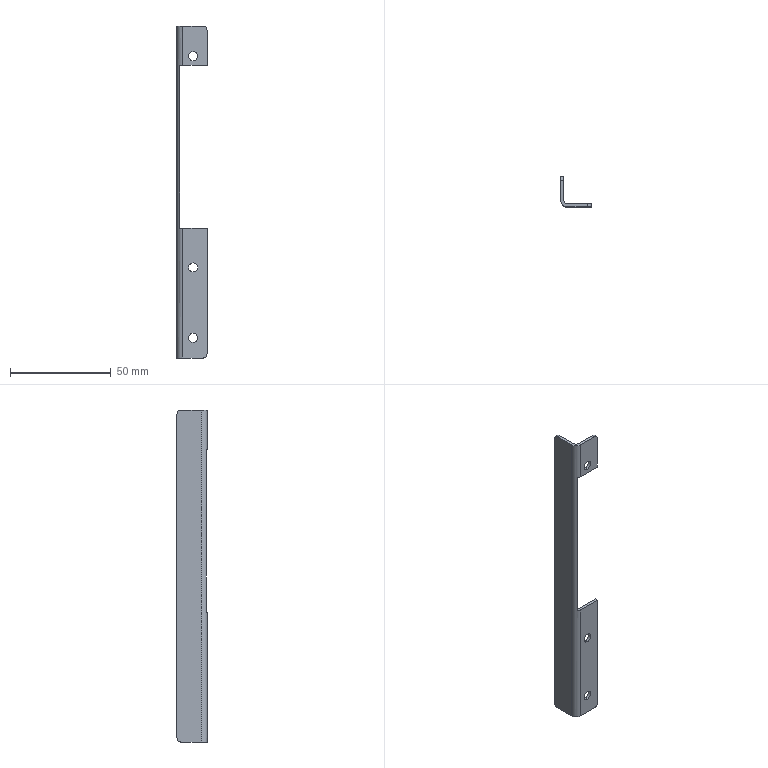Part | STEP file | 229H151431 Default | 1 solid | 26 faces | box 15 x 15 x 165 mm | volume 5074 mm3 | cylinder 13 | plane 13 | commonest cylinder face diameters 4.5 x6 4 x4 3 x2 6 x1
STEP:
#1=CARTESIAN_POINT('',(8.,0.,147.75));
#2=VERTEX_POINT('',#1);
#3=CARTESIAN_POINT('',(8.,0.,152.25));
#4=VERTEX_POINT('',#3);
#5=CARTESIAN_POINT('',(8.,0.,150.));
#6=DIRECTION('',(0.,1.,0.));
#7=DIRECTION('',(0.,0.,1.));
#8=AXIS2_PLACEMENT_3D('',#5,#6,#7);
#9=CIRCLE('',#8,2.25);
#10=EDGE_CURVE('',#2,#4,#9,.T.);
#11=ORIENTED_EDGE('',*,*,#10,.F.);
#12=CARTESIAN_POINT('',(8.,1.5,147.75));
#13=VERTEX_POINT('',#12);
#14=CARTESIAN_POINT('',(8.,-8.5,147.75));
#15=DIRECTION('',(0.,1.,0.));
#16=VECTOR('',#15,1000.);
#17=LINE('',#14,#16);
#18=EDGE_CURVE('',#2,#13,#17,.T.);
#19=ORIENTED_EDGE('',*,*,#18,.T.);
#20=CARTESIAN_POINT('',(8.,1.5,152.25));
#21=VERTEX_POINT('',#20);
#22=CARTESIAN_POINT('',(8.,1.5,150.));
#23=DIRECTION('',(0.,1.,0.));
#24=DIRECTION('',(0.,0.,1.));
#25=AXIS2_PLACEMENT_3D('',#22,#23,#24);
#26=CIRCLE('',#25,2.25);
#27=EDGE_CURVE('',#13,#21,#26,.T.);
#28=ORIENTED_EDGE('',*,*,#27,.T.);
#29=CARTESIAN_POINT('',(8.,-8.5,152.25));
#30=DIRECTION('',(0.,1.,0.));
#31=VECTOR('',#30,1000.);
#32=LINE('',#29,#31);
#33=EDGE_CURVE('',#4,#21,#32,.T.);
#34=ORIENTED_EDGE('',*,*,#33,.F.);
#35=EDGE_LOOP('',(#11,#19,#28,#34));
#36=FACE_OUTER_BOUND('',#35,.T.);
#37=CARTESIAN_POINT('',(8.,-8.5,150.));
#38=DIRECTION('',(0.,1.,0.));
#39=DIRECTION('',(0.,0.,1.));
#40=AXIS2_PLACEMENT_3D('',#37,#38,#39);
#41=CYLINDRICAL_SURFACE('',#40,2.25);
#42=ADVANCED_FACE('',(#36),#41,.F.);
#43=CARTESIAN_POINT('',(8.,0.,42.75));
#44=VERTEX_POINT('',#43);
#45=CARTESIAN_POINT('',(8.,0.,47.25));
#46=VERTEX_POINT('',#45);
#47=CARTESIAN_POINT('',(8.,0.,45.));
#48=DIRECTION('',(0.,1.,0.));
#49=DIRECTION('',(0.,0.,1.));
#50=AXIS2_PLACEMENT_3D('',#47,#48,#49);
#51=CIRCLE('',#50,2.25);
#52=EDGE_CURVE('',#44,#46,#51,.T.);
#53=ORIENTED_EDGE('',*,*,#52,.F.);
#54=CARTESIAN_POINT('',(8.,1.5,42.75));
#55=VERTEX_POINT('',#54);
#56=CARTESIAN_POINT('',(8.,-8.5,42.75));
#57=DIRECTION('',(0.,1.,0.));
#58=VECTOR('',#57,1000.);
#59=LINE('',#56,#58);
#60=EDGE_CURVE('',#44,#55,#59,.T.);
#61=ORIENTED_EDGE('',*,*,#60,.T.);
#62=CARTESIAN_POINT('',(8.,1.5,47.25));
#63=VERTEX_POINT('',#62);
#64=CARTESIAN_POINT('',(8.,1.5,45.));
#65=DIRECTION('',(0.,1.,0.));
#66=DIRECTION('',(0.,0.,1.));
#67=AXIS2_PLACEMENT_3D('',#64,#65,#66);
#68=CIRCLE('',#67,2.25);
#69=EDGE_CURVE('',#55,#63,#68,.T.);
#70=ORIENTED_EDGE('',*,*,#69,.T.);
#71=CARTESIAN_POINT('',(8.,-8.5,47.25));
#72=DIRECTION('',(0.,1.,0.));
#73=VECTOR('',#72,1000.);
#74=LINE('',#71,#73);
#75=EDGE_CURVE('',#46,#63,#74,.T.);
#76=ORIENTED_EDGE('',*,*,#75,.F.);
#77=EDGE_LOOP('',(#53,#61,#70,#76));
#78=FACE_OUTER_BOUND('',#77,.T.);
#79=CARTESIAN_POINT('',(8.,-8.5,45.));
#80=DIRECTION('',(0.,1.,0.));
#81=DIRECTION('',(0.,0.,1.));
#82=AXIS2_PLACEMENT_3D('',#79,#80,#81);
#83=CYLINDRICAL_SURFACE('',#82,2.25);
#84=ADVANCED_FACE('',(#78),#83,.F.);
#85=CARTESIAN_POINT('',(8.,0.,7.75));
#86=VERTEX_POINT('',#85);
#87=CARTESIAN_POINT('',(8.,0.,12.25));
#88=VERTEX_POINT('',#87);
#89=CARTESIAN_POINT('',(8.,0.,10.));
#90=DIRECTION('',(0.,1.,0.));
#91=DIRECTION('',(0.,0.,1.));
#92=AXIS2_PLACEMENT_3D('',#89,#90,#91);
#93=CIRCLE('',#92,2.25);
#94=EDGE_CURVE('',#86,#88,#93,.T.);
#95=ORIENTED_EDGE('',*,*,#94,.F.);
#96=CARTESIAN_POINT('',(8.,1.5,7.75));
#97=VERTEX_POINT('',#96);
#98=CARTESIAN_POINT('',(8.,-8.5,7.75));
#99=DIRECTION('',(0.,1.,0.));
#100=VECTOR('',#99,1000.);
#101=LINE('',#98,#100);
#102=EDGE_CURVE('',#86,#97,#101,.T.);
#103=ORIENTED_EDGE('',*,*,#102,.T.);
#104=CARTESIAN_POINT('',(8.,1.5,12.25));
#105=VERTEX_POINT('',#104);
#106=CARTESIAN_POINT('',(8.,1.5,10.));
#107=DIRECTION('',(0.,1.,0.));
#108=DIRECTION('',(0.,0.,1.));
#109=AXIS2_PLACEMENT_3D('',#106,#107,#108);
#110=CIRCLE('',#109,2.25);
#111=EDGE_CURVE('',#97,#105,#110,.T.);
#112=ORIENTED_EDGE('',*,*,#111,.T.);
#113=CARTESIAN_POINT('',(8.,-8.5,12.25));
#114=DIRECTION('',(0.,1.,0.));
#115=VECTOR('',#114,1000.);
#116=LINE('',#113,#115);
#117=EDGE_CURVE('',#88,#105,#116,.T.);
#118=ORIENTED_EDGE('',*,*,#117,.F.);
#119=EDGE_LOOP('',(#95,#103,#112,#118));
#120=FACE_OUTER_BOUND('',#119,.T.);
#121=CARTESIAN_POINT('',(8.,-8.5,10.));
#122=DIRECTION('',(0.,1.,0.));
#123=DIRECTION('',(0.,0.,1.));
#124=AXIS2_PLACEMENT_3D('',#121,#122,#123);
#125=CYLINDRICAL_SURFACE('',#124,2.25);
#126=ADVANCED_FACE('',(#120),#125,.F.);
#127=CARTESIAN_POINT('',(8.,0.,10.));
#128=DIRECTION('',(0.,1.,0.));
#129=DIRECTION('',(0.,0.,1.));
#130=AXIS2_PLACEMENT_3D('',#127,#128,#129);
#131=CIRCLE('',#130,2.25);
#132=EDGE_CURVE('',#88,#86,#131,.T.);
#133=ORIENTED_EDGE('',*,*,#132,.T.);
#134=ORIENTED_EDGE('',*,*,#94,.T.);
#135=EDGE_LOOP('',(#133,#134));
#136=FACE_BOUND('',#135,.T.);
#137=CARTESIAN_POINT('',(8.,0.,45.));
#138=DIRECTION('',(0.,1.,0.));
#139=DIRECTION('',(0.,0.,1.));
#140=AXIS2_PLACEMENT_3D('',#137,#138,#139);
#141=CIRCLE('',#140,2.25);
#142=EDGE_CURVE('',#46,#44,#141,.T.);
#143=ORIENTED_EDGE('',*,*,#142,.T.);
#144=ORIENTED_EDGE('',*,*,#52,.T.);
#145=EDGE_LOOP('',(#143,#144));
#146=FACE_BOUND('',#145,.T.);
#147=CARTESIAN_POINT('',(15.,0.,64.5));
#148=VERTEX_POINT('',#147);
#149=CARTESIAN_POINT('',(15.,0.,2.));
#150=VERTEX_POINT('',#149);
#151=CARTESIAN_POINT('',(15.,0.,165.));
#152=DIRECTION('',(0.,0.,-1.));
#153=VECTOR('',#152,1000.);
#154=LINE('',#151,#153);
#155=EDGE_CURVE('',#148,#150,#154,.T.);
#156=ORIENTED_EDGE('',*,*,#155,.F.);
#157=CARTESIAN_POINT('',(3.,0.,64.5));
#158=VERTEX_POINT('',#157);
#159=CARTESIAN_POINT('',(0.,0.,64.5));
#160=DIRECTION('',(-1.,0.,0.));
#161=VECTOR('',#160,1000.);
#162=LINE('',#159,#161);
#163=EDGE_CURVE('',#148,#158,#162,.T.);
#164=ORIENTED_EDGE('',*,*,#163,.T.);
#165=CARTESIAN_POINT('',(3.,0.,0.));
#166=VERTEX_POINT('',#165);
#167=CARTESIAN_POINT('',(3.,0.,165.));
#168=DIRECTION('',(0.,0.,-1.));
#169=VECTOR('',#168,1000.);
#170=LINE('',#167,#169);
#171=EDGE_CURVE('',#158,#166,#170,.T.);
#172=ORIENTED_EDGE('',*,*,#171,.T.);
#173=CARTESIAN_POINT('',(13.,0.,0.));
#174=VERTEX_POINT('',#173);
#175=CARTESIAN_POINT('',(0.,0.,0.));
#176=DIRECTION('',(1.,0.,0.));
#177=VECTOR('',#176,1000.);
#178=LINE('',#175,#177);
#179=EDGE_CURVE('',#166,#174,#178,.T.);
#180=ORIENTED_EDGE('',*,*,#179,.T.);
#181=CARTESIAN_POINT('',(13.,0.,2.));
#182=DIRECTION('',(0.,-1.,0.));
#183=DIRECTION('',(0.,0.,1.));
#184=AXIS2_PLACEMENT_3D('',#181,#182,#183);
#185=CIRCLE('',#184,2.);
#186=EDGE_CURVE('',#174,#150,#185,.T.);
#187=ORIENTED_EDGE('',*,*,#186,.T.);
#188=EDGE_LOOP('',(#156,#164,#172,#180,#187));
#189=FACE_OUTER_BOUND('',#188,.T.);
#190=CARTESIAN_POINT('',(0.,0.,165.));
#191=DIRECTION('',(0.,1.,0.));
#192=DIRECTION('',(0.,0.,1.));
#193=AXIS2_PLACEMENT_3D('',#190,#191,#192);
#194=PLANE('',#193);
#195=ADVANCED_FACE('',(#136,#146,#189),#194,.F.);
#196=CARTESIAN_POINT('',(15.,1.5,64.5));
#197=VERTEX_POINT('',#196);
#198=CARTESIAN_POINT('',(15.,1.5,2.));
#199=VERTEX_POINT('',#198);
#200=CARTESIAN_POINT('',(15.,1.5,165.));
#201=DIRECTION('',(0.,0.,-1.));
#202=VECTOR('',#201,1000.);
#203=LINE('',#200,#202);
#204=EDGE_CURVE('',#197,#199,#203,.T.);
#205=ORIENTED_EDGE('',*,*,#204,.F.);
#206=CARTESIAN_POINT('',(15.,1.5,64.5));
#207=DIRECTION('',(0.,-1.,0.));
#208=VECTOR('',#207,1000.);
#209=LINE('',#206,#208);
#210=EDGE_CURVE('',#197,#148,#209,.T.);
#211=ORIENTED_EDGE('',*,*,#210,.T.);
#212=ORIENTED_EDGE('',*,*,#155,.T.);
#213=CARTESIAN_POINT('',(15.,1.5,2.));
#214=DIRECTION('',(0.,1.,0.));
#215=VECTOR('',#214,1000.);
#216=LINE('',#213,#215);
#217=EDGE_CURVE('',#150,#199,#216,.T.);
#218=ORIENTED_EDGE('',*,*,#217,.T.);
#219=EDGE_LOOP('',(#205,#211,#212,#218));
#220=FACE_OUTER_BOUND('',#219,.T.);
#221=CARTESIAN_POINT('',(15.,1.5,165.));
#222=DIRECTION('',(-1.,0.,0.));
#223=DIRECTION('',(0.,0.,1.));
#224=AXIS2_PLACEMENT_3D('',#221,#222,#223);
#225=PLANE('',#224);
#226=ADVANCED_FACE('',(#220),#225,.F.);
#227=CARTESIAN_POINT('',(8.,1.5,10.));
#228=DIRECTION('',(0.,1.,0.));
#229=DIRECTION('',(0.,0.,1.));
#230=AXIS2_PLACEMENT_3D('',#227,#228,#229);
#231=CIRCLE('',#230,2.25);
#232=EDGE_CURVE('',#105,#97,#231,.T.);
#233=ORIENTED_EDGE('',*,*,#232,.F.);
#234=ORIENTED_EDGE('',*,*,#111,.F.);
#235=EDGE_LOOP('',(#233,#234));
#236=FACE_BOUND('',#235,.T.);
#237=CARTESIAN_POINT('',(8.,1.5,45.));
#238=DIRECTION('',(0.,1.,0.));
#239=DIRECTION('',(0.,0.,1.));
#240=AXIS2_PLACEMENT_3D('',#237,#238,#239);
#241=CIRCLE('',#240,2.25);
#242=EDGE_CURVE('',#63,#55,#241,.T.);
#243=ORIENTED_EDGE('',*,*,#242,.F.);
#244=ORIENTED_EDGE('',*,*,#69,.F.);
#245=EDGE_LOOP('',(#243,#244));
#246=FACE_BOUND('',#245,.T.);
#247=CARTESIAN_POINT('',(3.,1.5,0.));
#248=VERTEX_POINT('',#247);
#249=CARTESIAN_POINT('',(3.,1.5,64.5));
#250=VERTEX_POINT('',#249);
#251=CARTESIAN_POINT('',(3.,1.5,165.));
#252=DIRECTION('',(0.,0.,1.));
#253=VECTOR('',#252,1000.);
#254=LINE('',#251,#253);
#255=EDGE_CURVE('',#248,#250,#254,.T.);
#256=ORIENTED_EDGE('',*,*,#255,.T.);
#257=CARTESIAN_POINT('',(1.5,1.5,64.5));
#258=DIRECTION('',(1.,0.,0.));
#259=VECTOR('',#258,1000.);
#260=LINE('',#257,#259);
#261=EDGE_CURVE('',#250,#197,#260,.T.);
#262=ORIENTED_EDGE('',*,*,#261,.T.);
#263=ORIENTED_EDGE('',*,*,#204,.T.);
#264=CARTESIAN_POINT('',(13.,1.5,0.));
#265=VERTEX_POINT('',#264);
#266=CARTESIAN_POINT('',(13.,1.5,2.));
#267=DIRECTION('',(0.,1.,0.));
#268=DIRECTION('',(0.,0.,-1.));
#269=AXIS2_PLACEMENT_3D('',#266,#267,#268);
#270=CIRCLE('',#269,2.);
#271=EDGE_CURVE('',#199,#265,#270,.T.);
#272=ORIENTED_EDGE('',*,*,#271,.T.);
#273=CARTESIAN_POINT('',(1.5,1.5,0.));
#274=DIRECTION('',(-1.,0.,0.));
#275=VECTOR('',#274,1000.);
#276=LINE('',#273,#275);
#277=EDGE_CURVE('',#265,#248,#276,.T.);
#278=ORIENTED_EDGE('',*,*,#277,.T.);
#279=EDGE_LOOP('',(#256,#262,#263,#272,#278));
#280=FACE_OUTER_BOUND('',#279,.T.);
#281=CARTESIAN_POINT('',(1.5,1.5,165.));
#282=DIRECTION('',(0.,-1.,0.));
#283=DIRECTION('',(0.,0.,-1.));
#284=AXIS2_PLACEMENT_3D('',#281,#282,#283);
#285=PLANE('',#284);
#286=ADVANCED_FACE('',(#236,#246,#280),#285,.F.);
#287=CARTESIAN_POINT('',(1.5,3.,64.5));
#288=VERTEX_POINT('',#287);
#289=CARTESIAN_POINT('',(1.5,3.,0.));
#290=VERTEX_POINT('',#289);
#291=CARTESIAN_POINT('',(1.5,3.,0.));
#292=DIRECTION('',(0.,0.,-1.));
#293=VECTOR('',#292,1000.);
#294=LINE('',#291,#293);
#295=EDGE_CURVE('',#288,#290,#294,.T.);
#296=ORIENTED_EDGE('',*,*,#295,.F.);
#297=CARTESIAN_POINT('',(3.,3.,64.5));
#298=DIRECTION('',(0.,0.,1.));
#299=DIRECTION('',(-1.,0.,0.));
#300=AXIS2_PLACEMENT_3D('',#297,#298,#299);
#301=CIRCLE('',#300,1.5);
#302=EDGE_CURVE('',#288,#250,#301,.T.);
#303=ORIENTED_EDGE('',*,*,#302,.T.);
#304=ORIENTED_EDGE('',*,*,#255,.F.);
#305=CARTESIAN_POINT('',(3.,3.,0.));
#306=DIRECTION('',(0.,0.,1.));
#307=DIRECTION('',(1.,0.,0.));
#308=AXIS2_PLACEMENT_3D('',#305,#306,#307);
#309=CIRCLE('',#308,1.5);
#310=EDGE_CURVE('',#290,#248,#309,.T.);
#311=ORIENTED_EDGE('',*,*,#310,.F.);
#312=EDGE_LOOP('',(#296,#303,#304,#311));
#313=FACE_OUTER_BOUND('',#312,.T.);
#314=CARTESIAN_POINT('',(3.,3.,165.));
#315=DIRECTION('',(0.,0.,1.));
#316=DIRECTION('',(1.,0.,0.));
#317=AXIS2_PLACEMENT_3D('',#314,#315,#316);
#318=CYLINDRICAL_SURFACE('',#317,1.5);
#319=ADVANCED_FACE('',(#313),#318,.F.);
#320=CARTESIAN_POINT('',(1.5,15.,163.));
#321=VERTEX_POINT('',#320);
#322=CARTESIAN_POINT('',(1.5,15.,2.));
#323=VERTEX_POINT('',#322);
#324=CARTESIAN_POINT('',(1.5,15.,165.));
#325=DIRECTION('',(0.,0.,-1.));
#326=VECTOR('',#325,1000.);
#327=LINE('',#324,#326);
#328=EDGE_CURVE('',#321,#323,#327,.T.);
#329=ORIENTED_EDGE('',*,*,#328,.T.);
#330=CARTESIAN_POINT('',(0.,15.,2.));
#331=VERTEX_POINT('',#330);
#332=CARTESIAN_POINT('',(1.5,15.,2.));
#333=DIRECTION('',(-1.,0.,0.));
#334=VECTOR('',#333,1000.);
#335=LINE('',#332,#334);
#336=EDGE_CURVE('',#323,#331,#335,.T.);
#337=ORIENTED_EDGE('',*,*,#336,.T.);
#338=CARTESIAN_POINT('',(0.,15.,163.));
#339=VERTEX_POINT('',#338);
#340=CARTESIAN_POINT('',(0.,15.,165.));
#341=DIRECTION('',(0.,0.,-1.));
#342=VECTOR('',#341,1000.);
#343=LINE('',#340,#342);
#344=EDGE_CURVE('',#339,#331,#343,.T.);
#345=ORIENTED_EDGE('',*,*,#344,.F.);
#346=CARTESIAN_POINT('',(1.5,15.,163.));
#347=DIRECTION('',(1.,0.,0.));
#348=VECTOR('',#347,1000.);
#349=LINE('',#346,#348);
#350=EDGE_CURVE('',#339,#321,#349,.T.);
#351=ORIENTED_EDGE('',*,*,#350,.T.);
#352=EDGE_LOOP('',(#329,#337,#345,#351));
#353=FACE_OUTER_BOUND('',#352,.T.);
#354=CARTESIAN_POINT('',(1.5,15.,165.));
#355=DIRECTION('',(0.,-1.,0.));
#356=DIRECTION('',(0.,0.,-1.));
#357=AXIS2_PLACEMENT_3D('',#354,#355,#356);
#358=PLANE('',#357);
#359=ADVANCED_FACE('',(#353),#358,.F.);
#360=ORIENTED_EDGE('',*,*,#344,.T.);
#361=CARTESIAN_POINT('',(0.,13.,0.));
#362=VERTEX_POINT('',#361);
#363=CARTESIAN_POINT('',(0.,13.,2.));
#364=DIRECTION('',(-1.,0.,0.));
#365=DIRECTION('',(0.,1.,0.));
#366=AXIS2_PLACEMENT_3D('',#363,#364,#365);
#367=CIRCLE('',#366,2.);
#368=EDGE_CURVE('',#331,#362,#367,.T.);
#369=ORIENTED_EDGE('',*,*,#368,.T.);
#370=CARTESIAN_POINT('',(0.,3.,0.));
#371=VERTEX_POINT('',#370);
#372=CARTESIAN_POINT('',(0.,15.,0.));
#373=DIRECTION('',(0.,-1.,0.));
#374=VECTOR('',#373,1000.);
#375=LINE('',#372,#374);
#376=EDGE_CURVE('',#362,#371,#375,.T.);
#377=ORIENTED_EDGE('',*,*,#376,.T.);
#378=CARTESIAN_POINT('',(0.,3.,165.));
#379=VERTEX_POINT('',#378);
#380=CARTESIAN_POINT('',(0.,3.,165.));
#381=DIRECTION('',(0.,0.,1.));
#382=VECTOR('',#381,1000.);
#383=LINE('',#380,#382);
#384=EDGE_CURVE('',#371,#379,#383,.T.);
#385=ORIENTED_EDGE('',*,*,#384,.T.);
#386=CARTESIAN_POINT('',(0.,13.,165.));
#387=VERTEX_POINT('',#386);
#388=CARTESIAN_POINT('',(0.,15.,165.));
#389=DIRECTION('',(0.,-1.,0.));
#390=VECTOR('',#389,1000.);
#391=LINE('',#388,#390);
#392=EDGE_CURVE('',#387,#379,#391,.T.);
#393=ORIENTED_EDGE('',*,*,#392,.F.);
#394=CARTESIAN_POINT('',(0.,13.,163.));
#395=DIRECTION('',(-1.,0.,0.));
#396=DIRECTION('',(0.,1.,0.));
#397=AXIS2_PLACEMENT_3D('',#394,#395,#396);
#398=CIRCLE('',#397,2.);
#399=EDGE_CURVE('',#387,#339,#398,.T.);
#400=ORIENTED_EDGE('',*,*,#399,.T.);
#401=EDGE_LOOP('',(#360,#369,#377,#385,#393,#400));
#402=FACE_OUTER_BOUND('',#401,.T.);
#403=CARTESIAN_POINT('',(0.,15.,165.));
#404=DIRECTION('',(1.,0.,0.));
#405=DIRECTION('',(0.,1.,0.));
#406=AXIS2_PLACEMENT_3D('',#403,#404,#405);
#407=PLANE('',#406);
#408=ADVANCED_FACE('',(#402),#407,.F.);
#409=CARTESIAN_POINT('',(3.,0.,165.));
#410=VERTEX_POINT('',#409);
#411=CARTESIAN_POINT('',(3.,0.,145.5));
#412=VERTEX_POINT('',#411);
#413=CARTESIAN_POINT('',(3.,0.,165.));
#414=DIRECTION('',(0.,0.,-1.));
#415=VECTOR('',#414,1000.);
#416=LINE('',#413,#415);
#417=EDGE_CURVE('',#410,#412,#416,.T.);
#418=ORIENTED_EDGE('',*,*,#417,.T.);
#419=CARTESIAN_POINT('',(15.,0.,145.5));
#420=VERTEX_POINT('',#419);
#421=CARTESIAN_POINT('',(0.,0.,145.5));
#422=DIRECTION('',(1.,0.,0.));
#423=VECTOR('',#422,1000.);
#424=LINE('',#421,#423);
#425=EDGE_CURVE('',#412,#420,#424,.T.);
#426=ORIENTED_EDGE('',*,*,#425,.T.);
#427=CARTESIAN_POINT('',(15.,0.,163.));
#428=VERTEX_POINT('',#427);
#429=CARTESIAN_POINT('',(15.,0.,165.));
#430=DIRECTION('',(0.,0.,-1.));
#431=VECTOR('',#430,1000.);
#432=LINE('',#429,#431);
#433=EDGE_CURVE('',#428,#420,#432,.T.);
#434=ORIENTED_EDGE('',*,*,#433,.F.);
#435=CARTESIAN_POINT('',(13.,0.,165.));
#436=VERTEX_POINT('',#435);
#437=CARTESIAN_POINT('',(13.,0.,163.));
#438=DIRECTION('',(0.,-1.,0.));
#439=DIRECTION('',(0.,0.,1.));
#440=AXIS2_PLACEMENT_3D('',#437,#438,#439);
#441=CIRCLE('',#440,2.);
#442=EDGE_CURVE('',#428,#436,#441,.T.);
#443=ORIENTED_EDGE('',*,*,#442,.T.);
#444=CARTESIAN_POINT('',(0.,0.,165.));
#445=DIRECTION('',(1.,0.,0.));
#446=VECTOR('',#445,1000.);
#447=LINE('',#444,#446);
#448=EDGE_CURVE('',#410,#436,#447,.T.);
#449=ORIENTED_EDGE('',*,*,#448,.F.);
#450=EDGE_LOOP('',(#418,#426,#434,#443,#449));
#451=FACE_OUTER_BOUND('',#450,.T.);
#452=CARTESIAN_POINT('',(8.,0.,150.));
#453=DIRECTION('',(0.,1.,0.));
#454=DIRECTION('',(0.,0.,1.));
#455=AXIS2_PLACEMENT_3D('',#452,#453,#454);
#456=CIRCLE('',#455,2.25);
#457=EDGE_CURVE('',#4,#2,#456,.T.);
#458=ORIENTED_EDGE('',*,*,#457,.T.);
#459=ORIENTED_EDGE('',*,*,#10,.T.);
#460=EDGE_LOOP('',(#458,#459));
#461=FACE_BOUND('',#460,.T.);
#462=CARTESIAN_POINT('',(0.,0.,165.));
#463=DIRECTION('',(0.,1.,0.));
#464=DIRECTION('',(0.,0.,1.));
#465=AXIS2_PLACEMENT_3D('',#462,#463,#464);
#466=PLANE('',#465);
#467=ADVANCED_FACE('',(#451,#461),#466,.F.);
#468=ORIENTED_EDGE('',*,*,#433,.T.);
#469=CARTESIAN_POINT('',(15.,1.5,145.5));
#470=VERTEX_POINT('',#469);
#471=CARTESIAN_POINT('',(15.,1.5,145.5));
#472=DIRECTION('',(0.,1.,0.));
#473=VECTOR('',#472,1000.);
#474=LINE('',#471,#473);
#475=EDGE_CURVE('',#420,#470,#474,.T.);
#476=ORIENTED_EDGE('',*,*,#475,.T.);
#477=CARTESIAN_POINT('',(15.,1.5,163.));
#478=VERTEX_POINT('',#477);
#479=CARTESIAN_POINT('',(15.,1.5,165.));
#480=DIRECTION('',(0.,0.,-1.));
#481=VECTOR('',#480,1000.);
#482=LINE('',#479,#481);
#483=EDGE_CURVE('',#478,#470,#482,.T.);
#484=ORIENTED_EDGE('',*,*,#483,.F.);
#485=CARTESIAN_POINT('',(15.,0.,163.));
#486=DIRECTION('',(0.,-1.,0.));
#487=VECTOR('',#486,1000.);
#488=LINE('',#485,#487);
#489=EDGE_CURVE('',#478,#428,#488,.T.);
#490=ORIENTED_EDGE('',*,*,#489,.T.);
#491=EDGE_LOOP('',(#468,#476,#484,#490));
#492=FACE_OUTER_BOUND('',#491,.T.);
#493=CARTESIAN_POINT('',(15.,1.5,165.));
#494=DIRECTION('',(-1.,0.,0.));
#495=DIRECTION('',(0.,0.,1.));
#496=AXIS2_PLACEMENT_3D('',#493,#494,#495);
#497=PLANE('',#496);
#498=ADVANCED_FACE('',(#492),#497,.F.);
#499=ORIENTED_EDGE('',*,*,#483,.T.);
#500=CARTESIAN_POINT('',(3.,1.5,145.5));
#501=VERTEX_POINT('',#500);
#502=CARTESIAN_POINT('',(1.5,1.5,145.5));
#503=DIRECTION('',(-1.,0.,0.));
#504=VECTOR('',#503,1000.);
#505=LINE('',#502,#504);
#506=EDGE_CURVE('',#470,#501,#505,.T.);
#507=ORIENTED_EDGE('',*,*,#506,.T.);
#508=CARTESIAN_POINT('',(3.,1.5,165.));
#509=VERTEX_POINT('',#508);
#510=CARTESIAN_POINT('',(3.,1.5,165.));
#511=DIRECTION('',(0.,0.,1.));
#512=VECTOR('',#511,1000.);
#513=LINE('',#510,#512);
#514=EDGE_CURVE('',#501,#509,#513,.T.);
#515=ORIENTED_EDGE('',*,*,#514,.T.);
#516=CARTESIAN_POINT('',(13.,1.5,165.));
#517=VERTEX_POINT('',#516);
#518=CARTESIAN_POINT('',(1.5,1.5,165.));
#519=DIRECTION('',(-1.,0.,0.));
#520=VECTOR('',#519,1000.);
#521=LINE('',#518,#520);
#522=EDGE_CURVE('',#517,#509,#521,.T.);
#523=ORIENTED_EDGE('',*,*,#522,.F.);
#524=CARTESIAN_POINT('',(13.,1.5,163.));
#525=DIRECTION('',(0.,1.,0.));
#526=DIRECTION('',(0.,0.,-1.));
#527=AXIS2_PLACEMENT_3D('',#524,#525,#526);
#528=CIRCLE('',#527,2.);
#529=EDGE_CURVE('',#517,#478,#528,.T.);
#530=ORIENTED_EDGE('',*,*,#529,.T.);
#531=EDGE_LOOP('',(#499,#507,#515,#523,#530));
#532=FACE_OUTER_BOUND('',#531,.T.);
#533=CARTESIAN_POINT('',(8.,1.5,150.));
#534=DIRECTION('',(0.,1.,0.));
#535=DIRECTION('',(0.,0.,1.));
#536=AXIS2_PLACEMENT_3D('',#533,#534,#535);
#537=CIRCLE('',#536,2.25);
#538=EDGE_CURVE('',#21,#13,#537,.T.);
#539=ORIENTED_EDGE('',*,*,#538,.F.);
#540=ORIENTED_EDGE('',*,*,#27,.F.);
#541=EDGE_LOOP('',(#539,#540));
#542=FACE_BOUND('',#541,.T.);
#543=CARTESIAN_POINT('',(1.5,1.5,165.));
#544=DIRECTION('',(0.,-1.,0.));
#545=DIRECTION('',(0.,0.,-1.));
#546=AXIS2_PLACEMENT_3D('',#543,#544,#545);
#547=PLANE('',#546);
#548=ADVANCED_FACE('',(#532,#542),#547,.F.);
#549=CARTESIAN_POINT('',(1.5,3.,165.));
#550=VERTEX_POINT('',#549);
#551=CARTESIAN_POINT('',(1.5,3.,145.5));
#552=VERTEX_POINT('',#551);
#553=CARTESIAN_POINT('',(1.5,3.,0.));
#554=DIRECTION('',(0.,0.,-1.));
#555=VECTOR('',#554,1000.);
#556=LINE('',#553,#555);
#557=EDGE_CURVE('',#550,#552,#556,.T.);
#558=ORIENTED_EDGE('',*,*,#557,.T.);
#559=CARTESIAN_POINT('',(1.5,0.4019,145.5));
#560=VERTEX_POINT('',#559);
#561=CARTESIAN_POINT('',(1.5,-39.,145.5));
#562=DIRECTION('',(0.,1.,0.));
#563=VECTOR('',#562,1000.);
#564=LINE('',#561,#563);
#565=EDGE_CURVE('',#560,#552,#564,.T.);
#566=ORIENTED_EDGE('',*,*,#565,.F.);
#567=CARTESIAN_POINT('',(1.5,0.4019,64.5));
#568=VERTEX_POINT('',#567);
#569=CARTESIAN_POINT('',(1.5,0.4019,165.));
#570=DIRECTION('',(0.,0.,-1.));
#571=VECTOR('',#570,1000.);
#572=LINE('',#569,#571);
#573=EDGE_CURVE('',#560,#568,#572,.T.);
#574=ORIENTED_EDGE('',*,*,#573,.T.);
#575=CARTESIAN_POINT('',(1.5,-39.,64.5));
#576=DIRECTION('',(0.,1.,0.));
#577=VECTOR('',#576,1000.);
#578=LINE('',#575,#577);
#579=EDGE_CURVE('',#568,#288,#578,.T.);
#580=ORIENTED_EDGE('',*,*,#579,.T.);
#581=ORIENTED_EDGE('',*,*,#295,.T.);
#582=CARTESIAN_POINT('',(1.5,13.,0.));
#583=VERTEX_POINT('',#582);
#584=CARTESIAN_POINT('',(1.5,15.,0.));
#585=DIRECTION('',(0.,1.,0.));
#586=VECTOR('',#585,1000.);
#587=LINE('',#584,#586);
#588=EDGE_CURVE('',#290,#583,#587,.T.);
#589=ORIENTED_EDGE('',*,*,#588,.T.);
#590=CARTESIAN_POINT('',(1.5,13.,2.));
#591=DIRECTION('',(1.,0.,0.));
#592=DIRECTION('',(0.,-1.,0.));
#593=AXIS2_PLACEMENT_3D('',#590,#591,#592);
#594=CIRCLE('',#593,2.);
#595=EDGE_CURVE('',#583,#323,#594,.T.);
#596=ORIENTED_EDGE('',*,*,#595,.T.);
#597=ORIENTED_EDGE('',*,*,#328,.F.);
#598=CARTESIAN_POINT('',(1.5,13.,165.));
#599=VERTEX_POINT('',#598);
#600=CARTESIAN_POINT('',(1.5,13.,163.));
#601=DIRECTION('',(1.,0.,0.));
#602=DIRECTION('',(0.,-1.,0.));
#603=AXIS2_PLACEMENT_3D('',#600,#601,#602);
#604=CIRCLE('',#603,2.);
#605=EDGE_CURVE('',#321,#599,#604,.T.);
#606=ORIENTED_EDGE('',*,*,#605,.T.);
#607=CARTESIAN_POINT('',(1.5,15.,165.));
#608=DIRECTION('',(0.,1.,0.));
#609=VECTOR('',#608,1000.);
#610=LINE('',#607,#609);
#611=EDGE_CURVE('',#550,#599,#610,.T.);
#612=ORIENTED_EDGE('',*,*,#611,.F.);
#613=EDGE_LOOP('',(#558,#566,#574,#580,#581,#589,#596,#597,#606,#612));
#614=FACE_OUTER_BOUND('',#613,.T.);
#615=CARTESIAN_POINT('',(1.5,15.,165.));
#616=DIRECTION('',(-1.,0.,0.));
#617=DIRECTION('',(0.,-1.,0.));
#618=AXIS2_PLACEMENT_3D('',#615,#616,#617);
#619=PLANE('',#618);
#620=ADVANCED_FACE('',(#614),#619,.F.);
#621=ORIENTED_EDGE('',*,*,#448,.T.);
#622=CARTESIAN_POINT('',(13.,1.5,165.));
#623=DIRECTION('',(0.,1.,0.));
#624=VECTOR('',#623,1000.);
#625=LINE('',#622,#624);
#626=EDGE_CURVE('',#436,#517,#625,.T.);
#627=ORIENTED_EDGE('',*,*,#626,.T.);
#628=ORIENTED_EDGE('',*,*,#522,.T.);
#629=CARTESIAN_POINT('',(3.,3.,165.));
#630=DIRECTION('',(0.,0.,-1.));
#631=DIRECTION('',(1.,0.,0.));
#632=AXIS2_PLACEMENT_3D('',#629,#630,#631);
#633=CIRCLE('',#632,1.5);
#634=EDGE_CURVE('',#509,#550,#633,.T.);
#635=ORIENTED_EDGE('',*,*,#634,.T.);
#636=ORIENTED_EDGE('',*,*,#611,.T.);
#637=CARTESIAN_POINT('',(0.,13.,165.));
#638=DIRECTION('',(-1.,0.,0.));
#639=VECTOR('',#638,1000.);
#640=LINE('',#637,#639);
#641=EDGE_CURVE('',#599,#387,#640,.T.);
#642=ORIENTED_EDGE('',*,*,#641,.T.);
#643=ORIENTED_EDGE('',*,*,#392,.T.);
#644=CARTESIAN_POINT('',(3.,3.,165.));
#645=DIRECTION('',(0.,0.,1.));
#646=DIRECTION('',(1.,0.,0.));
#647=AXIS2_PLACEMENT_3D('',#644,#645,#646);
#648=CIRCLE('',#647,3.);
#649=EDGE_CURVE('',#379,#410,#648,.T.);
#650=ORIENTED_EDGE('',*,*,#649,.T.);
#651=EDGE_LOOP('',(#621,#627,#628,#635,#636,#642,#643,#650));
#652=FACE_OUTER_BOUND('',#651,.T.);
#653=CARTESIAN_POINT('',(0.,0.,165.));
#654=DIRECTION('',(0.,0.,1.));
#655=DIRECTION('',(1.,0.,0.));
#656=AXIS2_PLACEMENT_3D('',#653,#654,#655);
#657=PLANE('',#656);
#658=ADVANCED_FACE('',(#652),#657,.T.);
#659=ORIENTED_EDGE('',*,*,#277,.F.);
#660=CARTESIAN_POINT('',(13.,0.,0.));
#661=DIRECTION('',(0.,-1.,0.));
#662=VECTOR('',#661,1000.);
#663=LINE('',#660,#662);
#664=EDGE_CURVE('',#265,#174,#663,.T.);
#665=ORIENTED_EDGE('',*,*,#664,.T.);
#666=ORIENTED_EDGE('',*,*,#179,.F.);
#667=CARTESIAN_POINT('',(3.,3.,0.));
#668=DIRECTION('',(0.,0.,-1.));
#669=DIRECTION('',(1.,0.,0.));
#670=AXIS2_PLACEMENT_3D('',#667,#668,#669);
#671=CIRCLE('',#670,3.);
#672=EDGE_CURVE('',#166,#371,#671,.T.);
#673=ORIENTED_EDGE('',*,*,#672,.T.);
#674=ORIENTED_EDGE('',*,*,#376,.F.);
#675=CARTESIAN_POINT('',(0.,13.,0.));
#676=DIRECTION('',(1.,0.,0.));
#677=VECTOR('',#676,1000.);
#678=LINE('',#675,#677);
#679=EDGE_CURVE('',#362,#583,#678,.T.);
#680=ORIENTED_EDGE('',*,*,#679,.T.);
#681=ORIENTED_EDGE('',*,*,#588,.F.);
#682=ORIENTED_EDGE('',*,*,#310,.T.);
#683=EDGE_LOOP('',(#659,#665,#666,#673,#674,#680,#681,#682));
#684=FACE_OUTER_BOUND('',#683,.T.);
#685=CARTESIAN_POINT('',(0.,0.,0.));
#686=DIRECTION('',(0.,0.,1.));
#687=DIRECTION('',(1.,0.,0.));
#688=AXIS2_PLACEMENT_3D('',#685,#686,#687);
#689=PLANE('',#688);
#690=ADVANCED_FACE('',(#684),#689,.F.);
#691=ORIENTED_EDGE('',*,*,#514,.F.);
#692=CARTESIAN_POINT('',(3.,3.,145.5));
#693=DIRECTION('',(0.,0.,-1.));
#694=DIRECTION('',(1.,0.,0.));
#695=AXIS2_PLACEMENT_3D('',#692,#693,#694);
#696=CIRCLE('',#695,1.5);
#697=EDGE_CURVE('',#501,#552,#696,.T.);
#698=ORIENTED_EDGE('',*,*,#697,.T.);
#699=ORIENTED_EDGE('',*,*,#557,.F.);
#700=ORIENTED_EDGE('',*,*,#634,.F.);
#701=EDGE_LOOP('',(#691,#698,#699,#700));
#702=FACE_OUTER_BOUND('',#701,.T.);
#703=CARTESIAN_POINT('',(3.,3.,165.));
#704=DIRECTION('',(0.,0.,1.));
#705=DIRECTION('',(1.,0.,0.));
#706=AXIS2_PLACEMENT_3D('',#703,#704,#705);
#707=CYLINDRICAL_SURFACE('',#706,1.5);
#708=ADVANCED_FACE('',(#702),#707,.F.);
#709=CARTESIAN_POINT('',(3.,3.,64.5));
#710=DIRECTION('',(0.,0.,1.));
#711=DIRECTION('',(-1.,0.,0.));
#712=AXIS2_PLACEMENT_3D('',#709,#710,#711);
#713=CIRCLE('',#712,3.);
#714=EDGE_CURVE('',#568,#158,#713,.T.);
#715=ORIENTED_EDGE('',*,*,#714,.F.);
#716=ORIENTED_EDGE('',*,*,#573,.F.);
#717=CARTESIAN_POINT('',(3.,3.,145.5));
#718=DIRECTION('',(0.,0.,-1.));
#719=DIRECTION('',(1.,0.,0.));
#720=AXIS2_PLACEMENT_3D('',#717,#718,#719);
#721=CIRCLE('',#720,3.);
#722=EDGE_CURVE('',#412,#560,#721,.T.);
#723=ORIENTED_EDGE('',*,*,#722,.F.);
#724=ORIENTED_EDGE('',*,*,#417,.F.);
#725=ORIENTED_EDGE('',*,*,#649,.F.);
#726=ORIENTED_EDGE('',*,*,#384,.F.);
#727=ORIENTED_EDGE('',*,*,#672,.F.);
#728=ORIENTED_EDGE('',*,*,#171,.F.);
#729=EDGE_LOOP('',(#715,#716,#723,#724,#725,#726,#727,#728));
#730=FACE_OUTER_BOUND('',#729,.T.);
#731=CARTESIAN_POINT('',(3.,3.,165.));
#732=DIRECTION('',(0.,0.,-1.));
#733=DIRECTION('',(-1.,0.,0.));
#734=AXIS2_PLACEMENT_3D('',#731,#732,#733);
#735=CYLINDRICAL_SURFACE('',#734,3.);
#736=ADVANCED_FACE('',(#730),#735,.T.);
#737=ORIENTED_EDGE('',*,*,#442,.F.);
#738=ORIENTED_EDGE('',*,*,#489,.F.);
#739=ORIENTED_EDGE('',*,*,#529,.F.);
#740=ORIENTED_EDGE('',*,*,#626,.F.);
#741=EDGE_LOOP('',(#737,#738,#739,#740));
#742=FACE_OUTER_BOUND('',#741,.T.);
#743=CARTESIAN_POINT('',(13.,0.,163.));
#744=DIRECTION('',(0.,-1.,0.));
#745=DIRECTION('',(0.,0.,-1.));
#746=AXIS2_PLACEMENT_3D('',#743,#744,#745);
#747=CYLINDRICAL_SURFACE('',#746,2.);
#748=ADVANCED_FACE('',(#742),#747,.T.);
#749=ORIENTED_EDGE('',*,*,#186,.F.);
#750=ORIENTED_EDGE('',*,*,#664,.F.);
#751=ORIENTED_EDGE('',*,*,#271,.F.);
#752=ORIENTED_EDGE('',*,*,#217,.F.);
#753=EDGE_LOOP('',(#749,#750,#751,#752));
#754=FACE_OUTER_BOUND('',#753,.T.);
#755=CARTESIAN_POINT('',(13.,1.5,2.));
#756=DIRECTION('',(0.,1.,0.));
#757=DIRECTION('',(0.,0.,1.));
#758=AXIS2_PLACEMENT_3D('',#755,#756,#757);
#759=CYLINDRICAL_SURFACE('',#758,2.);
#760=ADVANCED_FACE('',(#754),#759,.T.);
#761=ORIENTED_EDGE('',*,*,#595,.F.);
#762=ORIENTED_EDGE('',*,*,#679,.F.);
#763=ORIENTED_EDGE('',*,*,#368,.F.);
#764=ORIENTED_EDGE('',*,*,#336,.F.);
#765=EDGE_LOOP('',(#761,#762,#763,#764));
#766=FACE_OUTER_BOUND('',#765,.T.);
#767=CARTESIAN_POINT('',(1.5,13.,2.));
#768=DIRECTION('',(-1.,0.,0.));
#769=DIRECTION('',(0.,0.,1.));
#770=AXIS2_PLACEMENT_3D('',#767,#768,#769);
#771=CYLINDRICAL_SURFACE('',#770,2.);
#772=ADVANCED_FACE('',(#766),#771,.T.);
#773=ORIENTED_EDGE('',*,*,#605,.F.);
#774=ORIENTED_EDGE('',*,*,#350,.F.);
#775=ORIENTED_EDGE('',*,*,#399,.F.);
#776=ORIENTED_EDGE('',*,*,#641,.F.);
#777=EDGE_LOOP('',(#773,#774,#775,#776));
#778=FACE_OUTER_BOUND('',#777,.T.);
#779=CARTESIAN_POINT('',(0.,13.,163.));
#780=DIRECTION('',(1.,0.,0.));
#781=DIRECTION('',(0.,0.,-1.));
#782=AXIS2_PLACEMENT_3D('',#779,#780,#781);
#783=CYLINDRICAL_SURFACE('',#782,2.);
#784=ADVANCED_FACE('',(#778),#783,.T.);
#785=ORIENTED_EDGE('',*,*,#102,.F.);
#786=ORIENTED_EDGE('',*,*,#132,.F.);
#787=ORIENTED_EDGE('',*,*,#117,.T.);
#788=ORIENTED_EDGE('',*,*,#232,.T.);
#789=EDGE_LOOP('',(#785,#786,#787,#788));
#790=FACE_OUTER_BOUND('',#789,.T.);
#791=CARTESIAN_POINT('',(8.,-8.5,10.));
#792=DIRECTION('',(0.,1.,0.));
#793=DIRECTION('',(0.,0.,1.));
#794=AXIS2_PLACEMENT_3D('',#791,#792,#793);
#795=CYLINDRICAL_SURFACE('',#794,2.25);
#796=ADVANCED_FACE('',(#790),#795,.F.);
#797=ORIENTED_EDGE('',*,*,#60,.F.);
#798=ORIENTED_EDGE('',*,*,#142,.F.);
#799=ORIENTED_EDGE('',*,*,#75,.T.);
#800=ORIENTED_EDGE('',*,*,#242,.T.);
#801=EDGE_LOOP('',(#797,#798,#799,#800));
#802=FACE_OUTER_BOUND('',#801,.T.);
#803=CARTESIAN_POINT('',(8.,-8.5,45.));
#804=DIRECTION('',(0.,1.,0.));
#805=DIRECTION('',(0.,0.,1.));
#806=AXIS2_PLACEMENT_3D('',#803,#804,#805);
#807=CYLINDRICAL_SURFACE('',#806,2.25);
#808=ADVANCED_FACE('',(#802),#807,.F.);
#809=ORIENTED_EDGE('',*,*,#18,.F.);
#810=ORIENTED_EDGE('',*,*,#457,.F.);
#811=ORIENTED_EDGE('',*,*,#33,.T.);
#812=ORIENTED_EDGE('',*,*,#538,.T.);
#813=EDGE_LOOP('',(#809,#810,#811,#812));
#814=FACE_OUTER_BOUND('',#813,.T.);
#815=CARTESIAN_POINT('',(8.,-8.5,150.));
#816=DIRECTION('',(0.,1.,0.));
#817=DIRECTION('',(0.,0.,1.));
#818=AXIS2_PLACEMENT_3D('',#815,#816,#817);
#819=CYLINDRICAL_SURFACE('',#818,2.25);
#820=ADVANCED_FACE('',(#814),#819,.F.);
#821=ORIENTED_EDGE('',*,*,#579,.F.);
#822=ORIENTED_EDGE('',*,*,#714,.T.);
#823=ORIENTED_EDGE('',*,*,#163,.F.);
#824=ORIENTED_EDGE('',*,*,#210,.F.);
#825=ORIENTED_EDGE('',*,*,#261,.F.);
#826=ORIENTED_EDGE('',*,*,#302,.F.);
#827=EDGE_LOOP('',(#821,#822,#823,#824,#825,#826));
#828=FACE_OUTER_BOUND('',#827,.T.);
#829=CARTESIAN_POINT('',(1.5,-39.,64.5));
#830=DIRECTION('',(0.,0.,-1.));
#831=DIRECTION('',(-1.,0.,0.));
#832=AXIS2_PLACEMENT_3D('',#829,#830,#831);
#833=PLANE('',#832);
#834=ADVANCED_FACE('',(#828),#833,.F.);
#835=ORIENTED_EDGE('',*,*,#506,.F.);
#836=ORIENTED_EDGE('',*,*,#475,.F.);
#837=ORIENTED_EDGE('',*,*,#425,.F.);
#838=ORIENTED_EDGE('',*,*,#722,.T.);
#839=ORIENTED_EDGE('',*,*,#565,.T.);
#840=ORIENTED_EDGE('',*,*,#697,.F.);
#841=EDGE_LOOP('',(#835,#836,#837,#838,#839,#840));
#842=FACE_OUTER_BOUND('',#841,.T.);
#843=CARTESIAN_POINT('',(1.5,-39.,145.5));
#844=DIRECTION('',(0.,0.,1.));
#845=DIRECTION('',(1.,0.,0.));
#846=AXIS2_PLACEMENT_3D('',#843,#844,#845);
#847=PLANE('',#846);
#848=ADVANCED_FACE('',(#842),#847,.F.);
#849=CLOSED_SHELL('',(#42,#84,#126,#195,#226,#286,#319,#359,#408,#467,#498,#548,#620,#658,#690,#708,#736,#748,#760,#772,#784,#796,#808,#820,#834,#848));
#850=MANIFOLD_SOLID_BREP('',#849);
#851=CARTESIAN_POINT('',(0.,0.,0.));
#852=DIRECTION('',(0.,0.,1.));
#853=DIRECTION('',(1.,0.,0.));
#854=AXIS2_PLACEMENT_3D('',#851,#852,#853);
#855=(LENGTH_UNIT()NAMED_UNIT(*)SI_UNIT(.MILLI.,.METRE.));
#856=UNCERTAINTY_MEASURE_WITH_UNIT(LENGTH_MEASURE(0.00001),#855,'','');
#857=(NAMED_UNIT(*)PLANE_ANGLE_UNIT()SI_UNIT($,.RADIAN.));
#858=(NAMED_UNIT(*)SI_UNIT($,.STERADIAN.)SOLID_ANGLE_UNIT());
#859=(GEOMETRIC_REPRESENTATION_CONTEXT(3)GLOBAL_UNCERTAINTY_ASSIGNED_CONTEXT((#856))GLOBAL_UNIT_ASSIGNED_CONTEXT((#855,#857,#858))REPRESENTATION_CONTEXT('',''));
#860=ADVANCED_BREP_SHAPE_REPRESENTATION('',(#850,#854),#859);